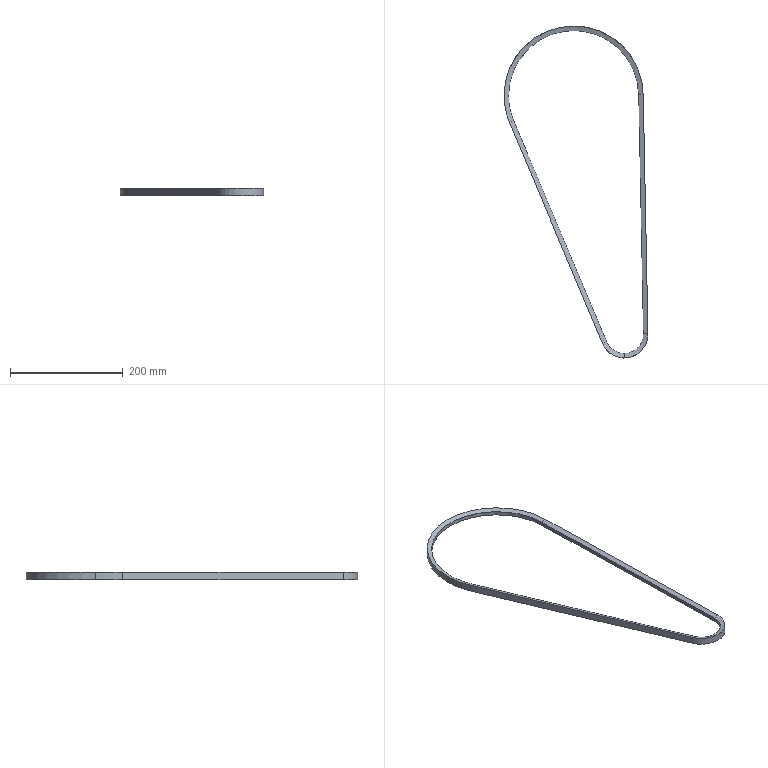Part | SolidWorks | features BaseBody 1 | 1 solid | 20 faces | box 255.391 x 589.134 x 12.57 mm | volume 105964 mm3 | plane 8 | cylinder 6 | cone 6 | commonest cylinder face diameters 231.15 x2 247.025 x2 68.168 x1 84.043 x1
STEP:
#1=CARTESIAN_POINT('',(-204.27,348.446,6.285));
#2=VERTEX_POINT('',#1);
#3=CARTESIAN_POINT('',(-213.941,396.356,6.285));
#4=VERTEX_POINT('',#3);
#5=CARTESIAN_POINT('',(-90.428,396.356,6.285));
#6=DIRECTION('',(0.,0.,-1.));
#7=DIRECTION('',(-1.,0.,0.));
#8=AXIS2_PLACEMENT_3D('',#5,#6,#7);
#9=CIRCLE('',#8,123.513);
#10=EDGE_CURVE('',#2,#4,#9,.T.);
#11=ORIENTED_EDGE('',*,*,#10,.T.);
#12=CARTESIAN_POINT('',(-213.941,396.356,-6.285));
#13=VERTEX_POINT('',#12);
#14=CARTESIAN_POINT('',(-213.941,396.356,0.));
#15=DIRECTION('',(0.,0.,-1.));
#16=VECTOR('',#15,1000.);
#17=LINE('',#14,#16);
#18=EDGE_CURVE('',#4,#13,#17,.T.);
#19=ORIENTED_EDGE('',*,*,#18,.T.);
#20=CARTESIAN_POINT('',(-204.27,348.446,-6.285));
#21=VERTEX_POINT('',#20);
#22=CARTESIAN_POINT('',(-90.428,396.356,-6.285));
#23=DIRECTION('',(0.,0.,1.));
#24=DIRECTION('',(-1.,0.,0.));
#25=AXIS2_PLACEMENT_3D('',#22,#23,#24);
#26=CIRCLE('',#25,123.513);
#27=EDGE_CURVE('',#13,#21,#26,.T.);
#28=ORIENTED_EDGE('',*,*,#27,.T.);
#29=CARTESIAN_POINT('',(-204.27,348.446,0.));
#30=DIRECTION('',(0.,0.,1.));
#31=VECTOR('',#30,1000.);
#32=LINE('',#29,#31);
#33=EDGE_CURVE('',#21,#2,#32,.T.);
#34=ORIENTED_EDGE('',*,*,#33,.T.);
#35=EDGE_LOOP('',(#11,#19,#28,#34));
#36=FACE_OUTER_BOUND('',#35,.T.);
#37=CARTESIAN_POINT('',(-90.428,396.356,0.));
#38=DIRECTION('',(0.,0.,-1.));
#39=DIRECTION('',(-1.,0.,0.));
#40=AXIS2_PLACEMENT_3D('',#37,#38,#39);
#41=CYLINDRICAL_SURFACE('',#40,123.513);
#42=ADVANCED_FACE('',(#36),#41,.T.);
#43=CARTESIAN_POINT('',(-90.428,511.931,-3.396));
#44=VERTEX_POINT('',#43);
#45=CARTESIAN_POINT('',(25.124,398.634,-3.396));
#46=VERTEX_POINT('',#45);
#47=CARTESIAN_POINT('',(-90.428,396.356,-3.396));
#48=DIRECTION('',(0.,0.,-1.));
#49=DIRECTION('',(-0.9998,-0.01971,0.));
#50=AXIS2_PLACEMENT_3D('',#47,#48,#49);
#51=CIRCLE('',#50,115.575);
#52=EDGE_CURVE('',#44,#46,#51,.T.);
#53=ORIENTED_EDGE('',*,*,#52,.F.);
#54=CARTESIAN_POINT('',(-90.428,519.869,-6.285));
#55=VERTEX_POINT('',#54);
#56=CARTESIAN_POINT('',(-90.428,519.869,-6.285));
#57=DIRECTION('',(0.,0.9397,-0.342));
#58=VECTOR('',#57,1000.);
#59=LINE('',#56,#58);
#60=EDGE_CURVE('',#44,#55,#59,.T.);
#61=ORIENTED_EDGE('',*,*,#60,.T.);
#62=CARTESIAN_POINT('',(33.06,398.79,-6.285));
#63=VERTEX_POINT('',#62);
#64=CARTESIAN_POINT('',(-90.428,396.356,-6.285));
#65=DIRECTION('',(0.,0.,1.));
#66=DIRECTION('',(-1.,0.,0.));
#67=AXIS2_PLACEMENT_3D('',#64,#65,#66);
#68=CIRCLE('',#67,123.513);
#69=EDGE_CURVE('',#63,#55,#68,.T.);
#70=ORIENTED_EDGE('',*,*,#69,.F.);
#71=CARTESIAN_POINT('',(29.092,398.712,-4.84));
#72=DIRECTION('',(0.9395,0.01852,-0.342));
#73=VECTOR('',#72,1000.);
#74=LINE('',#71,#73);
#75=EDGE_CURVE('',#46,#63,#74,.T.);
#76=ORIENTED_EDGE('',*,*,#75,.F.);
#77=EDGE_LOOP('',(#53,#61,#70,#76));
#78=FACE_OUTER_BOUND('',#77,.T.);
#79=CARTESIAN_POINT('',(-90.428,396.356,-6.285));
#80=DIRECTION('',(0.,0.,-1.));
#81=DIRECTION('',(0.,1.,0.));
#82=AXIS2_PLACEMENT_3D('',#79,#80,#81);
#83=CONICAL_SURFACE('',#82,123.513,1.222);
#84=ADVANCED_FACE('',(#78),#83,.F.);
#85=CARTESIAN_POINT('',(25.124,398.634,3.396));
#86=VERTEX_POINT('',#85);
#87=CARTESIAN_POINT('',(-206.003,396.356,3.396));
#88=VERTEX_POINT('',#87);
#89=CARTESIAN_POINT('',(-90.428,396.356,3.396));
#90=DIRECTION('',(0.,0.,1.));
#91=DIRECTION('',(-0.9998,-0.01971,0.));
#92=AXIS2_PLACEMENT_3D('',#89,#90,#91);
#93=CIRCLE('',#92,115.575);
#94=EDGE_CURVE('',#86,#88,#93,.T.);
#95=ORIENTED_EDGE('',*,*,#94,.T.);
#96=CARTESIAN_POINT('',(-206.003,396.356,-3.396));
#97=VERTEX_POINT('',#96);
#98=CARTESIAN_POINT('',(-206.003,396.356,0.));
#99=DIRECTION('',(0.,0.,-1.));
#100=VECTOR('',#99,1000.);
#101=LINE('',#98,#100);
#102=EDGE_CURVE('',#88,#97,#101,.T.);
#103=ORIENTED_EDGE('',*,*,#102,.T.);
#104=CARTESIAN_POINT('',(-90.428,396.356,-3.396));
#105=DIRECTION('',(0.,0.,-1.));
#106=DIRECTION('',(-0.9998,-0.01971,0.));
#107=AXIS2_PLACEMENT_3D('',#104,#105,#106);
#108=CIRCLE('',#107,115.575);
#109=EDGE_CURVE('',#97,#44,#108,.T.);
#110=ORIENTED_EDGE('',*,*,#109,.T.);
#111=ORIENTED_EDGE('',*,*,#52,.T.);
#112=CARTESIAN_POINT('',(25.124,398.634,0.));
#113=DIRECTION('',(0.,0.,-1.));
#114=VECTOR('',#113,1000.);
#115=LINE('',#112,#114);
#116=EDGE_CURVE('',#86,#46,#115,.T.);
#117=ORIENTED_EDGE('',*,*,#116,.F.);
#118=EDGE_LOOP('',(#95,#103,#110,#111,#117));
#119=FACE_OUTER_BOUND('',#118,.T.);
#120=CARTESIAN_POINT('',(-90.428,396.356,0.));
#121=DIRECTION('',(0.,0.,-1.));
#122=DIRECTION('',(-1.,0.,0.));
#123=AXIS2_PLACEMENT_3D('',#120,#121,#122);
#124=CYLINDRICAL_SURFACE('',#123,115.575);
#125=ADVANCED_FACE('',(#119),#124,.F.);
#126=CARTESIAN_POINT('',(-0.5712,-61.328,3.396));
#127=VERTEX_POINT('',#126);
#128=CARTESIAN_POINT('',(33.506,-26.572,3.396));
#129=VERTEX_POINT('',#128);
#130=CARTESIAN_POINT('',(-0.5712,-27.244,3.396));
#131=DIRECTION('',(0.,0.,1.));
#132=DIRECTION('',(0.9217,0.3879,0.));
#133=AXIS2_PLACEMENT_3D('',#130,#131,#132);
#134=CIRCLE('',#133,34.084);
#135=EDGE_CURVE('',#127,#129,#134,.T.);
#136=ORIENTED_EDGE('',*,*,#135,.F.);
#137=CARTESIAN_POINT('',(-0.5712,-69.265,6.285));
#138=VERTEX_POINT('',#137);
#139=CARTESIAN_POINT('',(-0.5712,-69.265,6.285));
#140=DIRECTION('',(0.,-0.9397,0.342));
#141=VECTOR('',#140,1000.);
#142=LINE('',#139,#141);
#143=EDGE_CURVE('',#127,#138,#142,.T.);
#144=ORIENTED_EDGE('',*,*,#143,.T.);
#145=CARTESIAN_POINT('',(41.442,-26.416,6.285));
#146=VERTEX_POINT('',#145);
#147=CARTESIAN_POINT('',(-0.5712,-27.244,6.285));
#148=DIRECTION('',(0.,0.,-1.));
#149=DIRECTION('',(-1.,0.,0.));
#150=AXIS2_PLACEMENT_3D('',#147,#148,#149);
#151=CIRCLE('',#150,42.021);
#152=EDGE_CURVE('',#146,#138,#151,.T.);
#153=ORIENTED_EDGE('',*,*,#152,.F.);
#154=CARTESIAN_POINT('',(33.506,-26.572,3.396));
#155=DIRECTION('',(0.9395,0.01852,0.342));
#156=VECTOR('',#155,1000.);
#157=LINE('',#154,#156);
#158=EDGE_CURVE('',#129,#146,#157,.T.);
#159=ORIENTED_EDGE('',*,*,#158,.F.);
#160=EDGE_LOOP('',(#136,#144,#153,#159));
#161=FACE_OUTER_BOUND('',#160,.T.);
#162=CARTESIAN_POINT('',(-0.5712,-27.244,6.285));
#163=DIRECTION('',(0.,0.,1.));
#164=DIRECTION('',(0.,-1.,0.));
#165=AXIS2_PLACEMENT_3D('',#162,#163,#164);
#166=CONICAL_SURFACE('',#165,42.021,1.222);
#167=ADVANCED_FACE('',(#161),#166,.F.);
#168=ORIENTED_EDGE('',*,*,#18,.F.);
#169=CARTESIAN_POINT('',(33.06,398.79,6.285));
#170=VERTEX_POINT('',#169);
#171=CARTESIAN_POINT('',(-90.428,396.356,6.285));
#172=DIRECTION('',(0.,0.,-1.));
#173=DIRECTION('',(-1.,0.,0.));
#174=AXIS2_PLACEMENT_3D('',#171,#172,#173);
#175=CIRCLE('',#174,123.513);
#176=EDGE_CURVE('',#4,#170,#175,.T.);
#177=ORIENTED_EDGE('',*,*,#176,.T.);
#178=CARTESIAN_POINT('',(33.06,398.79,0.));
#179=DIRECTION('',(0.,0.,-1.));
#180=VECTOR('',#179,1000.);
#181=LINE('',#178,#180);
#182=EDGE_CURVE('',#170,#63,#181,.T.);
#183=ORIENTED_EDGE('',*,*,#182,.T.);
#184=ORIENTED_EDGE('',*,*,#69,.T.);
#185=CARTESIAN_POINT('',(-90.428,396.356,-6.285));
#186=DIRECTION('',(0.,0.,1.));
#187=DIRECTION('',(-1.,0.,0.));
#188=AXIS2_PLACEMENT_3D('',#185,#186,#187);
#189=CIRCLE('',#188,123.513);
#190=EDGE_CURVE('',#55,#13,#189,.T.);
#191=ORIENTED_EDGE('',*,*,#190,.T.);
#192=EDGE_LOOP('',(#168,#177,#183,#184,#191));
#193=FACE_OUTER_BOUND('',#192,.T.);
#194=CARTESIAN_POINT('',(-90.428,396.356,0.));
#195=DIRECTION('',(0.,0.,-1.));
#196=DIRECTION('',(-1.,0.,0.));
#197=AXIS2_PLACEMENT_3D('',#194,#195,#196);
#198=CYLINDRICAL_SURFACE('',#197,123.513);
#199=ADVANCED_FACE('',(#193),#198,.T.);
#200=ORIENTED_EDGE('',*,*,#10,.F.);
#201=CARTESIAN_POINT('',(-196.954,351.525,3.396));
#202=VERTEX_POINT('',#201);
#203=CARTESIAN_POINT('',(-200.612,349.985,4.84));
#204=DIRECTION('',(-0.8661,-0.3645,0.342));
#205=VECTOR('',#204,1000.);
#206=LINE('',#203,#205);
#207=EDGE_CURVE('',#202,#2,#206,.T.);
#208=ORIENTED_EDGE('',*,*,#207,.F.);
#209=CARTESIAN_POINT('',(-90.428,396.356,3.396));
#210=DIRECTION('',(0.,0.,1.));
#211=DIRECTION('',(-0.9998,-0.01971,0.));
#212=AXIS2_PLACEMENT_3D('',#209,#210,#211);
#213=CIRCLE('',#212,115.575);
#214=EDGE_CURVE('',#88,#202,#213,.T.);
#215=ORIENTED_EDGE('',*,*,#214,.F.);
#216=ORIENTED_EDGE('',*,*,#94,.F.);
#217=CARTESIAN_POINT('',(29.092,398.712,4.84));
#218=DIRECTION('',(-0.9395,-0.01852,-0.342));
#219=VECTOR('',#218,1000.);
#220=LINE('',#217,#219);
#221=EDGE_CURVE('',#170,#86,#220,.T.);
#222=ORIENTED_EDGE('',*,*,#221,.F.);
#223=ORIENTED_EDGE('',*,*,#176,.F.);
#224=EDGE_LOOP('',(#200,#208,#215,#216,#222,#223));
#225=FACE_OUTER_BOUND('',#224,.T.);
#226=CARTESIAN_POINT('',(-90.428,396.356,6.285));
#227=DIRECTION('',(0.,0.,1.));
#228=DIRECTION('',(0.,-1.,0.));
#229=AXIS2_PLACEMENT_3D('',#226,#227,#228);
#230=CONICAL_SURFACE('',#229,123.513,1.222);
#231=ADVANCED_FACE('',(#225),#230,.F.);
#232=CARTESIAN_POINT('',(-39.302,-43.544,-6.285));
#233=VERTEX_POINT('',#232);
#234=CARTESIAN_POINT('',(-39.302,-43.544,6.285));
#235=VERTEX_POINT('',#234);
#236=CARTESIAN_POINT('',(-39.302,-43.544,6.285));
#237=DIRECTION('',(0.,0.,1.));
#238=VECTOR('',#237,1000.);
#239=LINE('',#236,#238);
#240=EDGE_CURVE('',#233,#235,#239,.T.);
#241=ORIENTED_EDGE('',*,*,#240,.T.);
#242=CARTESIAN_POINT('',(-39.302,-43.544,6.285));
#243=DIRECTION('',(-0.3879,0.9217,0.));
#244=VECTOR('',#243,1000.);
#245=LINE('',#242,#244);
#246=EDGE_CURVE('',#235,#2,#245,.T.);
#247=ORIENTED_EDGE('',*,*,#246,.T.);
#248=ORIENTED_EDGE('',*,*,#33,.F.);
#249=CARTESIAN_POINT('',(-39.302,-43.544,-6.285));
#250=DIRECTION('',(0.3879,-0.9217,0.));
#251=VECTOR('',#250,1000.);
#252=LINE('',#249,#251);
#253=EDGE_CURVE('',#21,#233,#252,.T.);
#254=ORIENTED_EDGE('',*,*,#253,.T.);
#255=EDGE_LOOP('',(#241,#247,#248,#254));
#256=FACE_OUTER_BOUND('',#255,.T.);
#257=CARTESIAN_POINT('',(-39.302,-43.544,6.285));
#258=DIRECTION('',(-0.9217,-0.3879,0.));
#259=DIRECTION('',(0.3879,-0.9217,0.));
#260=AXIS2_PLACEMENT_3D('',#257,#258,#259);
#261=PLANE('',#260);
#262=ADVANCED_FACE('',(#256),#261,.T.);
#263=ORIENTED_EDGE('',*,*,#60,.F.);
#264=ORIENTED_EDGE('',*,*,#109,.F.);
#265=CARTESIAN_POINT('',(-196.954,351.525,-3.396));
#266=VERTEX_POINT('',#265);
#267=CARTESIAN_POINT('',(-90.428,396.356,-3.396));
#268=DIRECTION('',(0.,0.,-1.));
#269=DIRECTION('',(-0.9998,-0.01971,0.));
#270=AXIS2_PLACEMENT_3D('',#267,#268,#269);
#271=CIRCLE('',#270,115.575);
#272=EDGE_CURVE('',#266,#97,#271,.T.);
#273=ORIENTED_EDGE('',*,*,#272,.F.);
#274=CARTESIAN_POINT('',(-200.612,349.985,-4.84));
#275=DIRECTION('',(0.8661,0.3645,0.342));
#276=VECTOR('',#275,1000.);
#277=LINE('',#274,#276);
#278=EDGE_CURVE('',#21,#266,#277,.T.);
#279=ORIENTED_EDGE('',*,*,#278,.F.);
#280=ORIENTED_EDGE('',*,*,#27,.F.);
#281=ORIENTED_EDGE('',*,*,#190,.F.);
#282=EDGE_LOOP('',(#263,#264,#273,#279,#280,#281));
#283=FACE_OUTER_BOUND('',#282,.T.);
#284=CARTESIAN_POINT('',(-90.428,396.356,-6.285));
#285=DIRECTION('',(0.,0.,-1.));
#286=DIRECTION('',(0.,1.,0.));
#287=AXIS2_PLACEMENT_3D('',#284,#285,#286);
#288=CONICAL_SURFACE('',#287,123.513,1.222);
#289=ADVANCED_FACE('',(#283),#288,.F.);
#290=ORIENTED_EDGE('',*,*,#182,.F.);
#291=CARTESIAN_POINT('',(33.06,398.79,6.285));
#292=DIRECTION('',(0.01971,-0.9998,0.));
#293=VECTOR('',#292,1000.);
#294=LINE('',#291,#293);
#295=EDGE_CURVE('',#170,#146,#294,.T.);
#296=ORIENTED_EDGE('',*,*,#295,.T.);
#297=CARTESIAN_POINT('',(41.442,-26.416,-6.285));
#298=VERTEX_POINT('',#297);
#299=CARTESIAN_POINT('',(41.442,-26.416,6.285));
#300=DIRECTION('',(0.,0.,-1.));
#301=VECTOR('',#300,1000.);
#302=LINE('',#299,#301);
#303=EDGE_CURVE('',#146,#298,#302,.T.);
#304=ORIENTED_EDGE('',*,*,#303,.T.);
#305=CARTESIAN_POINT('',(33.06,398.79,-6.285));
#306=DIRECTION('',(-0.01971,0.9998,0.));
#307=VECTOR('',#306,1000.);
#308=LINE('',#305,#307);
#309=EDGE_CURVE('',#298,#63,#308,.T.);
#310=ORIENTED_EDGE('',*,*,#309,.T.);
#311=EDGE_LOOP('',(#290,#296,#304,#310));
#312=FACE_OUTER_BOUND('',#311,.T.);
#313=CARTESIAN_POINT('',(33.06,398.79,6.285));
#314=DIRECTION('',(0.9998,0.01971,0.));
#315=DIRECTION('',(-0.01971,0.9998,0.));
#316=AXIS2_PLACEMENT_3D('',#313,#314,#315);
#317=PLANE('',#316);
#318=ADVANCED_FACE('',(#312),#317,.T.);
#319=ORIENTED_EDGE('',*,*,#221,.T.);
#320=CARTESIAN_POINT('',(25.124,398.634,3.396));
#321=DIRECTION('',(0.01971,-0.9998,0.));
#322=VECTOR('',#321,1000.);
#323=LINE('',#320,#322);
#324=EDGE_CURVE('',#86,#129,#323,.T.);
#325=ORIENTED_EDGE('',*,*,#324,.T.);
#326=ORIENTED_EDGE('',*,*,#158,.T.);
#327=ORIENTED_EDGE('',*,*,#295,.F.);
#328=EDGE_LOOP('',(#319,#325,#326,#327));
#329=FACE_OUTER_BOUND('',#328,.T.);
#330=CARTESIAN_POINT('',(25.124,398.634,3.396));
#331=DIRECTION('',(-0.342,-0.006741,0.9397));
#332=DIRECTION('',(0.9397,0.,0.342));
#333=AXIS2_PLACEMENT_3D('',#330,#331,#332);
#334=PLANE('',#333);
#335=ADVANCED_FACE('',(#329),#334,.T.);
#336=CARTESIAN_POINT('',(-31.986,-40.465,3.396));
#337=VERTEX_POINT('',#336);
#338=CARTESIAN_POINT('',(-39.302,-43.544,6.285));
#339=DIRECTION('',(0.8661,0.3645,-0.342));
#340=VECTOR('',#339,1000.);
#341=LINE('',#338,#340);
#342=EDGE_CURVE('',#235,#337,#341,.T.);
#343=ORIENTED_EDGE('',*,*,#342,.T.);
#344=CARTESIAN_POINT('',(-31.986,-40.465,3.396));
#345=DIRECTION('',(-0.3879,0.9217,0.));
#346=VECTOR('',#345,1000.);
#347=LINE('',#344,#346);
#348=EDGE_CURVE('',#337,#202,#347,.T.);
#349=ORIENTED_EDGE('',*,*,#348,.T.);
#350=ORIENTED_EDGE('',*,*,#207,.T.);
#351=ORIENTED_EDGE('',*,*,#246,.F.);
#352=EDGE_LOOP('',(#343,#349,#350,#351));
#353=FACE_OUTER_BOUND('',#352,.T.);
#354=CARTESIAN_POINT('',(-31.986,-40.465,3.396));
#355=DIRECTION('',(0.3152,0.1327,0.9397));
#356=DIRECTION('',(0.9481,0.,-0.3181));
#357=AXIS2_PLACEMENT_3D('',#354,#355,#356);
#358=PLANE('',#357);
#359=ADVANCED_FACE('',(#353),#358,.T.);
#360=ORIENTED_EDGE('',*,*,#102,.F.);
#361=ORIENTED_EDGE('',*,*,#214,.T.);
#362=CARTESIAN_POINT('',(-196.954,351.525,0.));
#363=DIRECTION('',(0.,0.,1.));
#364=VECTOR('',#363,1000.);
#365=LINE('',#362,#364);
#366=EDGE_CURVE('',#266,#202,#365,.T.);
#367=ORIENTED_EDGE('',*,*,#366,.F.);
#368=ORIENTED_EDGE('',*,*,#272,.T.);
#369=EDGE_LOOP('',(#360,#361,#367,#368));
#370=FACE_OUTER_BOUND('',#369,.T.);
#371=CARTESIAN_POINT('',(-90.428,396.356,0.));
#372=DIRECTION('',(0.,0.,-1.));
#373=DIRECTION('',(-1.,0.,0.));
#374=AXIS2_PLACEMENT_3D('',#371,#372,#373);
#375=CYLINDRICAL_SURFACE('',#374,115.575);
#376=ADVANCED_FACE('',(#370),#375,.F.);
#377=ORIENTED_EDGE('',*,*,#303,.F.);
#378=ORIENTED_EDGE('',*,*,#152,.T.);
#379=CARTESIAN_POINT('',(-0.5712,-27.244,6.285));
#380=DIRECTION('',(0.,0.,-1.));
#381=DIRECTION('',(-1.,0.,0.));
#382=AXIS2_PLACEMENT_3D('',#379,#380,#381);
#383=CIRCLE('',#382,42.021);
#384=EDGE_CURVE('',#138,#235,#383,.T.);
#385=ORIENTED_EDGE('',*,*,#384,.T.);
#386=ORIENTED_EDGE('',*,*,#240,.F.);
#387=CARTESIAN_POINT('',(-0.5712,-27.244,-6.285));
#388=DIRECTION('',(0.,0.,1.));
#389=DIRECTION('',(-1.,0.,0.));
#390=AXIS2_PLACEMENT_3D('',#387,#388,#389);
#391=CIRCLE('',#390,42.021);
#392=EDGE_CURVE('',#233,#298,#391,.T.);
#393=ORIENTED_EDGE('',*,*,#392,.T.);
#394=EDGE_LOOP('',(#377,#378,#385,#386,#393));
#395=FACE_OUTER_BOUND('',#394,.T.);
#396=CARTESIAN_POINT('',(-0.5712,-27.244,0.));
#397=DIRECTION('',(0.,0.,-1.));
#398=DIRECTION('',(-1.,0.,0.));
#399=AXIS2_PLACEMENT_3D('',#396,#397,#398);
#400=CYLINDRICAL_SURFACE('',#399,42.021);
#401=ADVANCED_FACE('',(#395),#400,.T.);
#402=CARTESIAN_POINT('',(-31.986,-40.465,-3.396));
#403=VERTEX_POINT('',#402);
#404=CARTESIAN_POINT('',(-31.986,-40.465,-3.396));
#405=DIRECTION('',(-0.8661,-0.3645,-0.342));
#406=VECTOR('',#405,1000.);
#407=LINE('',#404,#406);
#408=EDGE_CURVE('',#403,#233,#407,.T.);
#409=ORIENTED_EDGE('',*,*,#408,.T.);
#410=ORIENTED_EDGE('',*,*,#253,.F.);
#411=ORIENTED_EDGE('',*,*,#278,.T.);
#412=CARTESIAN_POINT('',(-196.954,351.525,-3.396));
#413=DIRECTION('',(0.3879,-0.9217,0.));
#414=VECTOR('',#413,1000.);
#415=LINE('',#412,#414);
#416=EDGE_CURVE('',#266,#403,#415,.T.);
#417=ORIENTED_EDGE('',*,*,#416,.T.);
#418=EDGE_LOOP('',(#409,#410,#411,#417));
#419=FACE_OUTER_BOUND('',#418,.T.);
#420=CARTESIAN_POINT('',(-39.302,-43.544,-6.285));
#421=DIRECTION('',(0.3152,0.1327,-0.9397));
#422=DIRECTION('',(-0.9481,0.,-0.3181));
#423=AXIS2_PLACEMENT_3D('',#420,#421,#422);
#424=PLANE('',#423);
#425=ADVANCED_FACE('',(#419),#424,.T.);
#426=ORIENTED_EDGE('',*,*,#75,.T.);
#427=ORIENTED_EDGE('',*,*,#309,.F.);
#428=CARTESIAN_POINT('',(33.506,-26.572,-3.396));
#429=VERTEX_POINT('',#428);
#430=CARTESIAN_POINT('',(41.442,-26.416,-6.285));
#431=DIRECTION('',(-0.9395,-0.01852,0.342));
#432=VECTOR('',#431,1000.);
#433=LINE('',#430,#432);
#434=EDGE_CURVE('',#298,#429,#433,.T.);
#435=ORIENTED_EDGE('',*,*,#434,.T.);
#436=CARTESIAN_POINT('',(33.506,-26.572,-3.396));
#437=DIRECTION('',(-0.01971,0.9998,0.));
#438=VECTOR('',#437,1000.);
#439=LINE('',#436,#438);
#440=EDGE_CURVE('',#429,#46,#439,.T.);
#441=ORIENTED_EDGE('',*,*,#440,.T.);
#442=EDGE_LOOP('',(#426,#427,#435,#441));
#443=FACE_OUTER_BOUND('',#442,.T.);
#444=CARTESIAN_POINT('',(33.06,398.79,-6.285));
#445=DIRECTION('',(-0.342,-0.006741,-0.9397));
#446=DIRECTION('',(-0.9397,0.,0.342));
#447=AXIS2_PLACEMENT_3D('',#444,#445,#446);
#448=PLANE('',#447);
#449=ADVANCED_FACE('',(#443),#448,.T.);
#450=ORIENTED_EDGE('',*,*,#116,.T.);
#451=ORIENTED_EDGE('',*,*,#440,.F.);
#452=CARTESIAN_POINT('',(33.506,-26.572,-3.396));
#453=DIRECTION('',(0.,0.,1.));
#454=VECTOR('',#453,1000.);
#455=LINE('',#452,#454);
#456=EDGE_CURVE('',#429,#129,#455,.T.);
#457=ORIENTED_EDGE('',*,*,#456,.T.);
#458=ORIENTED_EDGE('',*,*,#324,.F.);
#459=EDGE_LOOP('',(#450,#451,#457,#458));
#460=FACE_OUTER_BOUND('',#459,.T.);
#461=CARTESIAN_POINT('',(25.124,398.634,-3.396));
#462=DIRECTION('',(-0.9998,-0.01971,0.));
#463=DIRECTION('',(0.01971,-0.9998,0.));
#464=AXIS2_PLACEMENT_3D('',#461,#462,#463);
#465=PLANE('',#464);
#466=ADVANCED_FACE('',(#460),#465,.T.);
#467=ORIENTED_EDGE('',*,*,#143,.F.);
#468=CARTESIAN_POINT('',(-0.5712,-27.244,3.396));
#469=DIRECTION('',(0.,0.,1.));
#470=DIRECTION('',(0.9217,0.3879,0.));
#471=AXIS2_PLACEMENT_3D('',#468,#469,#470);
#472=CIRCLE('',#471,34.084);
#473=EDGE_CURVE('',#337,#127,#472,.T.);
#474=ORIENTED_EDGE('',*,*,#473,.F.);
#475=ORIENTED_EDGE('',*,*,#342,.F.);
#476=ORIENTED_EDGE('',*,*,#384,.F.);
#477=EDGE_LOOP('',(#467,#474,#475,#476));
#478=FACE_OUTER_BOUND('',#477,.T.);
#479=CARTESIAN_POINT('',(-0.5712,-27.244,6.285));
#480=DIRECTION('',(0.,0.,1.));
#481=DIRECTION('',(0.,-1.,0.));
#482=AXIS2_PLACEMENT_3D('',#479,#480,#481);
#483=CONICAL_SURFACE('',#482,42.021,1.222);
#484=ADVANCED_FACE('',(#478),#483,.F.);
#485=CARTESIAN_POINT('',(-31.986,-40.465,-3.396));
#486=DIRECTION('',(0.,0.,-1.));
#487=VECTOR('',#486,1000.);
#488=LINE('',#485,#487);
#489=EDGE_CURVE('',#337,#403,#488,.T.);
#490=ORIENTED_EDGE('',*,*,#489,.T.);
#491=ORIENTED_EDGE('',*,*,#416,.F.);
#492=ORIENTED_EDGE('',*,*,#366,.T.);
#493=ORIENTED_EDGE('',*,*,#348,.F.);
#494=EDGE_LOOP('',(#490,#491,#492,#493));
#495=FACE_OUTER_BOUND('',#494,.T.);
#496=CARTESIAN_POINT('',(-31.986,-40.465,-3.396));
#497=DIRECTION('',(0.9217,0.3879,0.));
#498=DIRECTION('',(-0.3879,0.9217,0.));
#499=AXIS2_PLACEMENT_3D('',#496,#497,#498);
#500=PLANE('',#499);
#501=ADVANCED_FACE('',(#495),#500,.T.);
#502=CARTESIAN_POINT('',(-0.5712,-27.244,-3.396));
#503=DIRECTION('',(0.,0.,-1.));
#504=DIRECTION('',(0.9217,0.3879,0.));
#505=AXIS2_PLACEMENT_3D('',#502,#503,#504);
#506=CIRCLE('',#505,34.084);
#507=EDGE_CURVE('',#429,#403,#506,.T.);
#508=ORIENTED_EDGE('',*,*,#507,.F.);
#509=ORIENTED_EDGE('',*,*,#434,.F.);
#510=ORIENTED_EDGE('',*,*,#392,.F.);
#511=ORIENTED_EDGE('',*,*,#408,.F.);
#512=EDGE_LOOP('',(#508,#509,#510,#511));
#513=FACE_OUTER_BOUND('',#512,.T.);
#514=CARTESIAN_POINT('',(-0.5712,-27.244,-6.285));
#515=DIRECTION('',(0.,0.,-1.));
#516=DIRECTION('',(-1.,0.,0.));
#517=AXIS2_PLACEMENT_3D('',#514,#515,#516);
#518=CONICAL_SURFACE('',#517,42.021,1.222);
#519=ADVANCED_FACE('',(#513),#518,.F.);
#520=ORIENTED_EDGE('',*,*,#473,.T.);
#521=ORIENTED_EDGE('',*,*,#135,.T.);
#522=ORIENTED_EDGE('',*,*,#456,.F.);
#523=ORIENTED_EDGE('',*,*,#507,.T.);
#524=ORIENTED_EDGE('',*,*,#489,.F.);
#525=EDGE_LOOP('',(#520,#521,#522,#523,#524));
#526=FACE_OUTER_BOUND('',#525,.T.);
#527=CARTESIAN_POINT('',(-0.5712,-27.244,0.));
#528=DIRECTION('',(0.,0.,-1.));
#529=DIRECTION('',(-1.,0.,0.));
#530=AXIS2_PLACEMENT_3D('',#527,#528,#529);
#531=CYLINDRICAL_SURFACE('',#530,34.084);
#532=ADVANCED_FACE('',(#526),#531,.F.);
#533=CLOSED_SHELL('',(#42,#84,#125,#167,#199,#231,#262,#289,#318,#335,#359,#376,#401,#425,#449,#466,#484,#501,#519,#532));
#534=MANIFOLD_SOLID_BREP('',#533);
#535=CARTESIAN_POINT('',(0.,0.,0.));
#536=DIRECTION('',(0.,0.,1.));
#537=DIRECTION('',(1.,0.,0.));
#538=AXIS2_PLACEMENT_3D('',#535,#536,#537);
#539=(LENGTH_UNIT()NAMED_UNIT(*)SI_UNIT(.MILLI.,.METRE.));
#540=UNCERTAINTY_MEASURE_WITH_UNIT(LENGTH_MEASURE(0.00001),#539,'','');
#541=(NAMED_UNIT(*)PLANE_ANGLE_UNIT()SI_UNIT($,.RADIAN.));
#542=(NAMED_UNIT(*)SI_UNIT($,.STERADIAN.)SOLID_ANGLE_UNIT());
#543=(GEOMETRIC_REPRESENTATION_CONTEXT(3)GLOBAL_UNCERTAINTY_ASSIGNED_CONTEXT((#540))GLOBAL_UNIT_ASSIGNED_CONTEXT((#539,#541,#542))REPRESENTATION_CONTEXT('',''));
#544=ADVANCED_BREP_SHAPE_REPRESENTATION('',(#534,#538),#543);